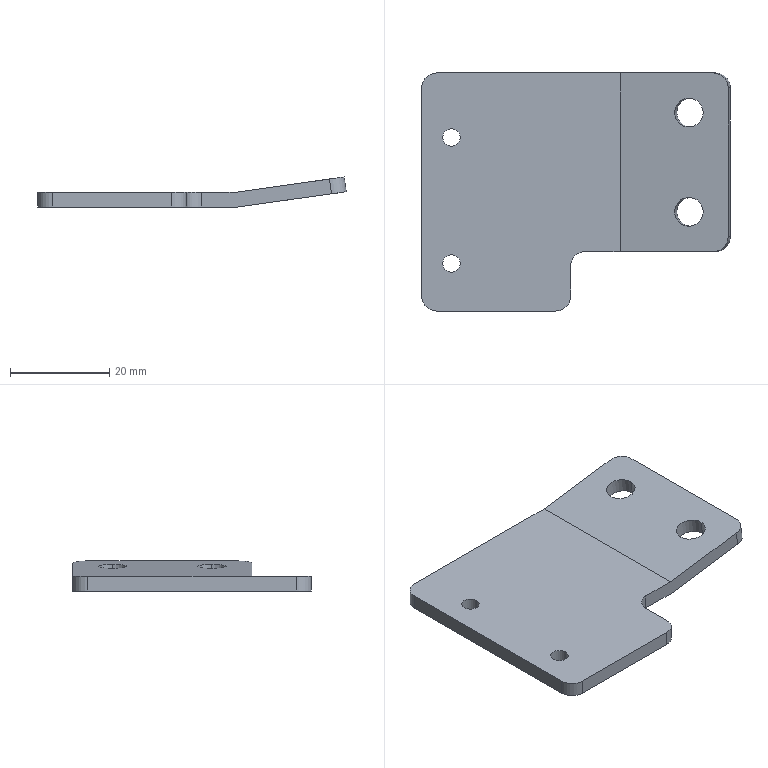Part | STEP file | J014-EBZ05-21-06 | 1 solid | 24 faces | box 62.203 x 48 x 6.062 mm | volume 7559 mm3 | cylinder 14 | plane 10 | commonest cylinder face diameters 6 x6 3.5 x4 5.8 x4
STEP:
#1=CARTESIAN_POINT('',(50.992,20.,4.545));
#2=VERTEX_POINT('',#1);
#3=CARTESIAN_POINT('',(56.736,20.,5.352));
#4=VERTEX_POINT('',#3);
#5=CARTESIAN_POINT('',(53.864,20.,4.948));
#6=DIRECTION('',(0.1392,0.,-0.9903));
#7=DIRECTION('',(0.9903,0.,0.1392));
#8=AXIS2_PLACEMENT_3D('',#5,#6,#7);
#9=CIRCLE('',#8,2.9);
#10=EDGE_CURVE('',#2,#4,#9,.T.);
#11=ORIENTED_EDGE('',*,*,#10,.F.);
#12=CARTESIAN_POINT('',(51.409,20.,1.574));
#13=VERTEX_POINT('',#12);
#14=CARTESIAN_POINT('',(50.992,20.,4.545));
#15=DIRECTION('',(0.1392,0.,-0.9903));
#16=VECTOR('',#15,1000.);
#17=LINE('',#14,#16);
#18=EDGE_CURVE('',#2,#13,#17,.T.);
#19=ORIENTED_EDGE('',*,*,#18,.T.);
#20=CARTESIAN_POINT('',(57.153,20.,2.381));
#21=VERTEX_POINT('',#20);
#22=CARTESIAN_POINT('',(54.281,20.,1.978));
#23=DIRECTION('',(-0.1392,0.,0.9903));
#24=DIRECTION('',(-0.9903,0.,-0.1392));
#25=AXIS2_PLACEMENT_3D('',#22,#23,#24);
#26=CIRCLE('',#25,2.9);
#27=EDGE_CURVE('',#21,#13,#26,.T.);
#28=ORIENTED_EDGE('',*,*,#27,.F.);
#29=CARTESIAN_POINT('',(56.736,20.,5.352));
#30=DIRECTION('',(0.1392,0.,-0.9903));
#31=VECTOR('',#30,1000.);
#32=LINE('',#29,#31);
#33=EDGE_CURVE('',#4,#21,#32,.T.);
#34=ORIENTED_EDGE('',*,*,#33,.F.);
#35=EDGE_LOOP('',(#11,#19,#28,#34));
#36=FACE_OUTER_BOUND('',#35,.T.);
#37=CARTESIAN_POINT('',(53.864,20.,4.948));
#38=DIRECTION('',(0.1392,0.,-0.9903));
#39=DIRECTION('',(0.9903,0.,0.1392));
#40=AXIS2_PLACEMENT_3D('',#37,#38,#39);
#41=CYLINDRICAL_SURFACE('',#40,2.9);
#42=ADVANCED_FACE('',(#36),#41,.F.);
#43=CARTESIAN_POINT('',(50.992,40.,4.545));
#44=VERTEX_POINT('',#43);
#45=CARTESIAN_POINT('',(56.736,40.,5.352));
#46=VERTEX_POINT('',#45);
#47=CARTESIAN_POINT('',(53.864,40.,4.948));
#48=DIRECTION('',(0.1392,0.,-0.9903));
#49=DIRECTION('',(0.9903,0.,0.1392));
#50=AXIS2_PLACEMENT_3D('',#47,#48,#49);
#51=CIRCLE('',#50,2.9);
#52=EDGE_CURVE('',#44,#46,#51,.T.);
#53=ORIENTED_EDGE('',*,*,#52,.F.);
#54=CARTESIAN_POINT('',(51.409,40.,1.574));
#55=VERTEX_POINT('',#54);
#56=CARTESIAN_POINT('',(50.992,40.,4.545));
#57=DIRECTION('',(0.1392,0.,-0.9903));
#58=VECTOR('',#57,1000.);
#59=LINE('',#56,#58);
#60=EDGE_CURVE('',#44,#55,#59,.T.);
#61=ORIENTED_EDGE('',*,*,#60,.T.);
#62=CARTESIAN_POINT('',(57.153,40.,2.381));
#63=VERTEX_POINT('',#62);
#64=CARTESIAN_POINT('',(54.281,40.,1.978));
#65=DIRECTION('',(-0.1392,0.,0.9903));
#66=DIRECTION('',(-0.9903,0.,-0.1392));
#67=AXIS2_PLACEMENT_3D('',#64,#65,#66);
#68=CIRCLE('',#67,2.9);
#69=EDGE_CURVE('',#63,#55,#68,.T.);
#70=ORIENTED_EDGE('',*,*,#69,.F.);
#71=CARTESIAN_POINT('',(56.736,40.,5.352));
#72=DIRECTION('',(0.1392,0.,-0.9903));
#73=VECTOR('',#72,1000.);
#74=LINE('',#71,#73);
#75=EDGE_CURVE('',#46,#63,#74,.T.);
#76=ORIENTED_EDGE('',*,*,#75,.F.);
#77=EDGE_LOOP('',(#53,#61,#70,#76));
#78=FACE_OUTER_BOUND('',#77,.T.);
#79=CARTESIAN_POINT('',(53.864,40.,4.948));
#80=DIRECTION('',(0.1392,0.,-0.9903));
#81=DIRECTION('',(0.9903,0.,0.1392));
#82=AXIS2_PLACEMENT_3D('',#79,#80,#81);
#83=CYLINDRICAL_SURFACE('',#82,2.9);
#84=ADVANCED_FACE('',(#78),#83,.F.);
#85=CARTESIAN_POINT('',(4.25,9.6,3.));
#86=VERTEX_POINT('',#85);
#87=CARTESIAN_POINT('',(7.75,9.6,3.));
#88=VERTEX_POINT('',#87);
#89=CARTESIAN_POINT('',(6.,9.6,3.));
#90=DIRECTION('',(0.,0.,-1.));
#91=DIRECTION('',(1.,0.,0.));
#92=AXIS2_PLACEMENT_3D('',#89,#90,#91);
#93=CIRCLE('',#92,1.75);
#94=EDGE_CURVE('',#86,#88,#93,.T.);
#95=ORIENTED_EDGE('',*,*,#94,.F.);
#96=CARTESIAN_POINT('',(4.25,9.6,0.));
#97=VERTEX_POINT('',#96);
#98=CARTESIAN_POINT('',(4.25,9.6,3.));
#99=DIRECTION('',(0.,0.,-1.));
#100=VECTOR('',#99,1000.);
#101=LINE('',#98,#100);
#102=EDGE_CURVE('',#86,#97,#101,.T.);
#103=ORIENTED_EDGE('',*,*,#102,.T.);
#104=CARTESIAN_POINT('',(7.75,9.6,0.));
#105=VERTEX_POINT('',#104);
#106=CARTESIAN_POINT('',(6.,9.6,0.));
#107=DIRECTION('',(0.,0.,1.));
#108=DIRECTION('',(-1.,0.,0.));
#109=AXIS2_PLACEMENT_3D('',#106,#107,#108);
#110=CIRCLE('',#109,1.75);
#111=EDGE_CURVE('',#105,#97,#110,.T.);
#112=ORIENTED_EDGE('',*,*,#111,.F.);
#113=CARTESIAN_POINT('',(7.75,9.6,3.));
#114=DIRECTION('',(0.,0.,-1.));
#115=VECTOR('',#114,1000.);
#116=LINE('',#113,#115);
#117=EDGE_CURVE('',#88,#105,#116,.T.);
#118=ORIENTED_EDGE('',*,*,#117,.F.);
#119=EDGE_LOOP('',(#95,#103,#112,#118));
#120=FACE_OUTER_BOUND('',#119,.T.);
#121=CARTESIAN_POINT('',(6.,9.6,3.));
#122=DIRECTION('',(0.,0.,-1.));
#123=DIRECTION('',(1.,0.,0.));
#124=AXIS2_PLACEMENT_3D('',#121,#122,#123);
#125=CYLINDRICAL_SURFACE('',#124,1.75);
#126=ADVANCED_FACE('',(#120),#125,.F.);
#127=CARTESIAN_POINT('',(4.25,35.,3.));
#128=VERTEX_POINT('',#127);
#129=CARTESIAN_POINT('',(7.75,35.,3.));
#130=VERTEX_POINT('',#129);
#131=CARTESIAN_POINT('',(6.,35.,3.));
#132=DIRECTION('',(0.,0.,-1.));
#133=DIRECTION('',(1.,0.,0.));
#134=AXIS2_PLACEMENT_3D('',#131,#132,#133);
#135=CIRCLE('',#134,1.75);
#136=EDGE_CURVE('',#128,#130,#135,.T.);
#137=ORIENTED_EDGE('',*,*,#136,.F.);
#138=CARTESIAN_POINT('',(4.25,35.,0.));
#139=VERTEX_POINT('',#138);
#140=CARTESIAN_POINT('',(4.25,35.,3.));
#141=DIRECTION('',(0.,0.,-1.));
#142=VECTOR('',#141,1000.);
#143=LINE('',#140,#142);
#144=EDGE_CURVE('',#128,#139,#143,.T.);
#145=ORIENTED_EDGE('',*,*,#144,.T.);
#146=CARTESIAN_POINT('',(7.75,35.,0.));
#147=VERTEX_POINT('',#146);
#148=CARTESIAN_POINT('',(6.,35.,0.));
#149=DIRECTION('',(0.,0.,1.));
#150=DIRECTION('',(-1.,0.,0.));
#151=AXIS2_PLACEMENT_3D('',#148,#149,#150);
#152=CIRCLE('',#151,1.75);
#153=EDGE_CURVE('',#147,#139,#152,.T.);
#154=ORIENTED_EDGE('',*,*,#153,.F.);
#155=CARTESIAN_POINT('',(7.75,35.,3.));
#156=DIRECTION('',(0.,0.,-1.));
#157=VECTOR('',#156,1000.);
#158=LINE('',#155,#157);
#159=EDGE_CURVE('',#130,#147,#158,.T.);
#160=ORIENTED_EDGE('',*,*,#159,.F.);
#161=EDGE_LOOP('',(#137,#145,#154,#160));
#162=FACE_OUTER_BOUND('',#161,.T.);
#163=CARTESIAN_POINT('',(6.,35.,3.));
#164=DIRECTION('',(0.,0.,-1.));
#165=DIRECTION('',(1.,0.,0.));
#166=AXIS2_PLACEMENT_3D('',#163,#164,#165);
#167=CYLINDRICAL_SURFACE('',#166,1.75);
#168=ADVANCED_FACE('',(#162),#167,.F.);
#169=CARTESIAN_POINT('',(61.786,45.,6.062));
#170=VERTEX_POINT('',#169);
#171=CARTESIAN_POINT('',(61.786,15.,6.062));
#172=VERTEX_POINT('',#171);
#173=CARTESIAN_POINT('',(61.786,24.,6.062));
#174=DIRECTION('',(0.,-1.,0.));
#175=VECTOR('',#174,1000.);
#176=LINE('',#173,#175);
#177=EDGE_CURVE('',#170,#172,#176,.T.);
#178=ORIENTED_EDGE('',*,*,#177,.T.);
#179=CARTESIAN_POINT('',(62.203,15.,3.091));
#180=VERTEX_POINT('',#179);
#181=CARTESIAN_POINT('',(62.203,15.,3.091));
#182=DIRECTION('',(0.1392,0.,-0.9903));
#183=VECTOR('',#182,1000.);
#184=LINE('',#181,#183);
#185=EDGE_CURVE('',#172,#180,#184,.T.);
#186=ORIENTED_EDGE('',*,*,#185,.T.);
#187=CARTESIAN_POINT('',(62.203,45.,3.091));
#188=VERTEX_POINT('',#187);
#189=CARTESIAN_POINT('',(62.203,24.,3.091));
#190=DIRECTION('',(0.,1.,0.));
#191=VECTOR('',#190,1000.);
#192=LINE('',#189,#191);
#193=EDGE_CURVE('',#180,#188,#192,.T.);
#194=ORIENTED_EDGE('',*,*,#193,.T.);
#195=CARTESIAN_POINT('',(61.786,45.,6.062));
#196=DIRECTION('',(-0.1392,0.,0.9903));
#197=VECTOR('',#196,1000.);
#198=LINE('',#195,#197);
#199=EDGE_CURVE('',#188,#170,#198,.T.);
#200=ORIENTED_EDGE('',*,*,#199,.T.);
#201=EDGE_LOOP('',(#178,#186,#194,#200));
#202=FACE_OUTER_BOUND('',#201,.T.);
#203=CARTESIAN_POINT('',(61.786,24.,6.062));
#204=DIRECTION('',(0.9903,0.,0.1392));
#205=DIRECTION('',(-0.1392,0.,0.9903));
#206=AXIS2_PLACEMENT_3D('',#203,#204,#205);
#207=PLANE('',#206);
#208=ADVANCED_FACE('',(#202),#207,.T.);
#209=ORIENTED_EDGE('',*,*,#193,.F.);
#210=CARTESIAN_POINT('',(59.233,12.,2.673));
#211=VERTEX_POINT('',#210);
#212=CARTESIAN_POINT('',(59.233,15.,2.673));
#213=DIRECTION('',(0.1392,0.,-0.9903));
#214=DIRECTION('',(0.,-1.,0.));
#215=AXIS2_PLACEMENT_3D('',#212,#213,#214);
#216=CIRCLE('',#215,3.);
#217=EDGE_CURVE('',#180,#211,#216,.T.);
#218=ORIENTED_EDGE('',*,*,#217,.T.);
#219=CARTESIAN_POINT('',(40.21,12.,0.));
#220=VERTEX_POINT('',#219);
#221=CARTESIAN_POINT('',(50.32,12.,1.421));
#222=DIRECTION('',(0.9903,0.,0.1392));
#223=VECTOR('',#222,1000.);
#224=LINE('',#221,#223);
#225=EDGE_CURVE('',#220,#211,#224,.T.);
#226=ORIENTED_EDGE('',*,*,#225,.F.);
#227=CARTESIAN_POINT('',(40.21,48.,0.));
#228=VERTEX_POINT('',#227);
#229=CARTESIAN_POINT('',(40.21,24.,0.));
#230=DIRECTION('',(0.,1.,0.));
#231=VECTOR('',#230,1000.);
#232=LINE('',#229,#231);
#233=EDGE_CURVE('',#220,#228,#232,.T.);
#234=ORIENTED_EDGE('',*,*,#233,.T.);
#235=CARTESIAN_POINT('',(59.233,48.,2.673));
#236=VERTEX_POINT('',#235);
#237=CARTESIAN_POINT('',(50.32,48.,1.421));
#238=DIRECTION('',(-0.9903,0.,-0.1392));
#239=VECTOR('',#238,1000.);
#240=LINE('',#237,#239);
#241=EDGE_CURVE('',#236,#228,#240,.T.);
#242=ORIENTED_EDGE('',*,*,#241,.F.);
#243=CARTESIAN_POINT('',(59.233,45.,2.673));
#244=DIRECTION('',(0.1392,0.,-0.9903));
#245=DIRECTION('',(0.,-1.,0.));
#246=AXIS2_PLACEMENT_3D('',#243,#244,#245);
#247=CIRCLE('',#246,3.);
#248=EDGE_CURVE('',#236,#188,#247,.T.);
#249=ORIENTED_EDGE('',*,*,#248,.T.);
#250=EDGE_LOOP('',(#209,#218,#226,#234,#242,#249));
#251=FACE_OUTER_BOUND('',#250,.T.);
#252=ORIENTED_EDGE('',*,*,#27,.T.);
#253=CARTESIAN_POINT('',(54.281,20.,1.978));
#254=DIRECTION('',(-0.1392,0.,0.9903));
#255=DIRECTION('',(-0.9903,0.,-0.1392));
#256=AXIS2_PLACEMENT_3D('',#253,#254,#255);
#257=CIRCLE('',#256,2.9);
#258=EDGE_CURVE('',#13,#21,#257,.T.);
#259=ORIENTED_EDGE('',*,*,#258,.T.);
#260=EDGE_LOOP('',(#252,#259));
#261=FACE_BOUND('',#260,.T.);
#262=ORIENTED_EDGE('',*,*,#69,.T.);
#263=CARTESIAN_POINT('',(54.281,40.,1.978));
#264=DIRECTION('',(-0.1392,0.,0.9903));
#265=DIRECTION('',(-0.9903,0.,-0.1392));
#266=AXIS2_PLACEMENT_3D('',#263,#264,#265);
#267=CIRCLE('',#266,2.9);
#268=EDGE_CURVE('',#55,#63,#267,.T.);
#269=ORIENTED_EDGE('',*,*,#268,.T.);
#270=EDGE_LOOP('',(#262,#269));
#271=FACE_BOUND('',#270,.T.);
#272=CARTESIAN_POINT('',(50.32,24.,1.421));
#273=DIRECTION('',(0.1392,0.,-0.9903));
#274=DIRECTION('',(0.,-1.,0.));
#275=AXIS2_PLACEMENT_3D('',#272,#273,#274);
#276=PLANE('',#275);
#277=ADVANCED_FACE('',(#251,#261,#271),#276,.T.);
#278=CARTESIAN_POINT('',(3.,48.,0.));
#279=VERTEX_POINT('',#278);
#280=CARTESIAN_POINT('',(49.903,48.,0.));
#281=DIRECTION('',(-1.,0.,0.));
#282=VECTOR('',#281,1000.);
#283=LINE('',#280,#282);
#284=EDGE_CURVE('',#228,#279,#283,.T.);
#285=ORIENTED_EDGE('',*,*,#284,.T.);
#286=CARTESIAN_POINT('',(3.,48.,3.));
#287=VERTEX_POINT('',#286);
#288=CARTESIAN_POINT('',(3.,48.,4.392));
#289=DIRECTION('',(0.,0.,1.));
#290=VECTOR('',#289,1000.);
#291=LINE('',#288,#290);
#292=EDGE_CURVE('',#279,#287,#291,.T.);
#293=ORIENTED_EDGE('',*,*,#292,.T.);
#294=CARTESIAN_POINT('',(40.,48.,3.));
#295=VERTEX_POINT('',#294);
#296=CARTESIAN_POINT('',(20.,48.,3.));
#297=DIRECTION('',(1.,0.,0.));
#298=VECTOR('',#297,1000.);
#299=LINE('',#296,#298);
#300=EDGE_CURVE('',#287,#295,#299,.T.);
#301=ORIENTED_EDGE('',*,*,#300,.T.);
#302=CARTESIAN_POINT('',(58.815,48.,5.644));
#303=VERTEX_POINT('',#302);
#304=CARTESIAN_POINT('',(49.903,48.,4.392));
#305=DIRECTION('',(0.9903,0.,0.1392));
#306=VECTOR('',#305,1000.);
#307=LINE('',#304,#306);
#308=EDGE_CURVE('',#295,#303,#307,.T.);
#309=ORIENTED_EDGE('',*,*,#308,.T.);
#310=CARTESIAN_POINT('',(58.815,48.,5.644));
#311=DIRECTION('',(0.1392,0.,-0.9903));
#312=VECTOR('',#311,1000.);
#313=LINE('',#310,#312);
#314=EDGE_CURVE('',#303,#236,#313,.T.);
#315=ORIENTED_EDGE('',*,*,#314,.T.);
#316=ORIENTED_EDGE('',*,*,#241,.T.);
#317=EDGE_LOOP('',(#285,#293,#301,#309,#315,#316));
#318=FACE_OUTER_BOUND('',#317,.T.);
#319=CARTESIAN_POINT('',(49.903,48.,4.392));
#320=DIRECTION('',(0.,1.,0.));
#321=DIRECTION('',(0.1392,0.,-0.9903));
#322=AXIS2_PLACEMENT_3D('',#319,#320,#321);
#323=PLANE('',#322);
#324=ADVANCED_FACE('',(#318),#323,.T.);
#325=CARTESIAN_POINT('',(3.,0.,0.));
#326=VERTEX_POINT('',#325);
#327=CARTESIAN_POINT('',(27.,0.,0.));
#328=VERTEX_POINT('',#327);
#329=CARTESIAN_POINT('',(49.903,0.,0.));
#330=DIRECTION('',(1.,0.,0.));
#331=VECTOR('',#330,1000.);
#332=LINE('',#329,#331);
#333=EDGE_CURVE('',#326,#328,#332,.T.);
#334=ORIENTED_EDGE('',*,*,#333,.T.);
#335=CARTESIAN_POINT('',(27.,0.,3.));
#336=VERTEX_POINT('',#335);
#337=CARTESIAN_POINT('',(27.,0.,3.));
#338=DIRECTION('',(0.,0.,1.));
#339=VECTOR('',#338,1000.);
#340=LINE('',#337,#339);
#341=EDGE_CURVE('',#328,#336,#340,.T.);
#342=ORIENTED_EDGE('',*,*,#341,.T.);
#343=CARTESIAN_POINT('',(3.,0.,3.));
#344=VERTEX_POINT('',#343);
#345=CARTESIAN_POINT('',(20.,0.,3.));
#346=DIRECTION('',(-1.,0.,0.));
#347=VECTOR('',#346,1000.);
#348=LINE('',#345,#347);
#349=EDGE_CURVE('',#336,#344,#348,.T.);
#350=ORIENTED_EDGE('',*,*,#349,.T.);
#351=CARTESIAN_POINT('',(3.,0.,4.392));
#352=DIRECTION('',(0.,0.,-1.));
#353=VECTOR('',#352,1000.);
#354=LINE('',#351,#353);
#355=EDGE_CURVE('',#344,#326,#354,.T.);
#356=ORIENTED_EDGE('',*,*,#355,.T.);
#357=EDGE_LOOP('',(#334,#342,#350,#356));
#358=FACE_OUTER_BOUND('',#357,.T.);
#359=CARTESIAN_POINT('',(49.903,0.,4.392));
#360=DIRECTION('',(0.,-1.,0.));
#361=DIRECTION('',(-0.1392,0.,0.9903));
#362=AXIS2_PLACEMENT_3D('',#359,#360,#361);
#363=PLANE('',#362);
#364=ADVANCED_FACE('',(#358),#363,.T.);
#365=CARTESIAN_POINT('',(58.815,12.,5.644));
#366=VERTEX_POINT('',#365);
#367=CARTESIAN_POINT('',(40.,12.,3.));
#368=VERTEX_POINT('',#367);
#369=CARTESIAN_POINT('',(49.903,12.,4.392));
#370=DIRECTION('',(-0.9903,0.,-0.1392));
#371=VECTOR('',#370,1000.);
#372=LINE('',#369,#371);
#373=EDGE_CURVE('',#366,#368,#372,.T.);
#374=ORIENTED_EDGE('',*,*,#373,.F.);
#375=CARTESIAN_POINT('',(58.815,15.,5.644));
#376=DIRECTION('',(-0.1392,0.,0.9903));
#377=DIRECTION('',(0.,1.,0.));
#378=AXIS2_PLACEMENT_3D('',#375,#376,#377);
#379=CIRCLE('',#378,3.);
#380=EDGE_CURVE('',#366,#172,#379,.T.);
#381=ORIENTED_EDGE('',*,*,#380,.T.);
#382=ORIENTED_EDGE('',*,*,#177,.F.);
#383=CARTESIAN_POINT('',(58.815,45.,5.644));
#384=DIRECTION('',(-0.1392,0.,0.9903));
#385=DIRECTION('',(0.,1.,0.));
#386=AXIS2_PLACEMENT_3D('',#383,#384,#385);
#387=CIRCLE('',#386,3.);
#388=EDGE_CURVE('',#170,#303,#387,.T.);
#389=ORIENTED_EDGE('',*,*,#388,.T.);
#390=ORIENTED_EDGE('',*,*,#308,.F.);
#391=CARTESIAN_POINT('',(40.,24.,3.));
#392=DIRECTION('',(0.,-1.,0.));
#393=VECTOR('',#392,1000.);
#394=LINE('',#391,#393);
#395=EDGE_CURVE('',#295,#368,#394,.T.);
#396=ORIENTED_EDGE('',*,*,#395,.T.);
#397=EDGE_LOOP('',(#374,#381,#382,#389,#390,#396));
#398=FACE_OUTER_BOUND('',#397,.T.);
#399=CARTESIAN_POINT('',(53.864,20.,4.948));
#400=DIRECTION('',(0.1392,0.,-0.9903));
#401=DIRECTION('',(0.9903,0.,0.1392));
#402=AXIS2_PLACEMENT_3D('',#399,#400,#401);
#403=CIRCLE('',#402,2.9);
#404=EDGE_CURVE('',#4,#2,#403,.T.);
#405=ORIENTED_EDGE('',*,*,#404,.T.);
#406=ORIENTED_EDGE('',*,*,#10,.T.);
#407=EDGE_LOOP('',(#405,#406));
#408=FACE_BOUND('',#407,.T.);
#409=CARTESIAN_POINT('',(53.864,40.,4.948));
#410=DIRECTION('',(0.1392,0.,-0.9903));
#411=DIRECTION('',(0.9903,0.,0.1392));
#412=AXIS2_PLACEMENT_3D('',#409,#410,#411);
#413=CIRCLE('',#412,2.9);
#414=EDGE_CURVE('',#46,#44,#413,.T.);
#415=ORIENTED_EDGE('',*,*,#414,.T.);
#416=ORIENTED_EDGE('',*,*,#52,.T.);
#417=EDGE_LOOP('',(#415,#416));
#418=FACE_BOUND('',#417,.T.);
#419=CARTESIAN_POINT('',(49.903,24.,4.392));
#420=DIRECTION('',(-0.1392,0.,0.9903));
#421=DIRECTION('',(0.,1.,0.));
#422=AXIS2_PLACEMENT_3D('',#419,#420,#421);
#423=PLANE('',#422);
#424=ADVANCED_FACE('',(#398,#408,#418),#423,.T.);
#425=CARTESIAN_POINT('',(30.,3.,0.));
#426=VERTEX_POINT('',#425);
#427=CARTESIAN_POINT('',(30.,9.,0.));
#428=VERTEX_POINT('',#427);
#429=CARTESIAN_POINT('',(30.,59.004,0.));
#430=DIRECTION('',(0.,1.,0.));
#431=VECTOR('',#430,1000.);
#432=LINE('',#429,#431);
#433=EDGE_CURVE('',#426,#428,#432,.T.);
#434=ORIENTED_EDGE('',*,*,#433,.F.);
#435=CARTESIAN_POINT('',(27.,3.,0.));
#436=DIRECTION('',(0.,0.,-1.));
#437=DIRECTION('',(1.,0.,0.));
#438=AXIS2_PLACEMENT_3D('',#435,#436,#437);
#439=CIRCLE('',#438,3.);
#440=EDGE_CURVE('',#426,#328,#439,.T.);
#441=ORIENTED_EDGE('',*,*,#440,.T.);
#442=ORIENTED_EDGE('',*,*,#333,.F.);
#443=CARTESIAN_POINT('',(0.,3.,0.));
#444=VERTEX_POINT('',#443);
#445=CARTESIAN_POINT('',(3.,3.,0.));
#446=DIRECTION('',(0.,0.,-1.));
#447=DIRECTION('',(1.,0.,0.));
#448=AXIS2_PLACEMENT_3D('',#445,#446,#447);
#449=CIRCLE('',#448,3.);
#450=EDGE_CURVE('',#326,#444,#449,.T.);
#451=ORIENTED_EDGE('',*,*,#450,.T.);
#452=CARTESIAN_POINT('',(0.,45.,0.));
#453=VERTEX_POINT('',#452);
#454=CARTESIAN_POINT('',(0.,24.,0.));
#455=DIRECTION('',(0.,-1.,0.));
#456=VECTOR('',#455,1000.);
#457=LINE('',#454,#456);
#458=EDGE_CURVE('',#453,#444,#457,.T.);
#459=ORIENTED_EDGE('',*,*,#458,.F.);
#460=CARTESIAN_POINT('',(3.,45.,0.));
#461=DIRECTION('',(0.,0.,-1.));
#462=DIRECTION('',(1.,0.,0.));
#463=AXIS2_PLACEMENT_3D('',#460,#461,#462);
#464=CIRCLE('',#463,3.);
#465=EDGE_CURVE('',#453,#279,#464,.T.);
#466=ORIENTED_EDGE('',*,*,#465,.T.);
#467=ORIENTED_EDGE('',*,*,#284,.F.);
#468=ORIENTED_EDGE('',*,*,#233,.F.);
#469=CARTESIAN_POINT('',(33.,12.,0.));
#470=VERTEX_POINT('',#469);
#471=CARTESIAN_POINT('',(55.128,12.,0.));
#472=DIRECTION('',(1.,0.,0.));
#473=VECTOR('',#472,1000.);
#474=LINE('',#471,#473);
#475=EDGE_CURVE('',#470,#220,#474,.T.);
#476=ORIENTED_EDGE('',*,*,#475,.F.);
#477=CARTESIAN_POINT('',(33.,9.,0.));
#478=DIRECTION('',(0.,0.,1.));
#479=DIRECTION('',(1.,0.,0.));
#480=AXIS2_PLACEMENT_3D('',#477,#478,#479);
#481=CIRCLE('',#480,3.);
#482=EDGE_CURVE('',#470,#428,#481,.T.);
#483=ORIENTED_EDGE('',*,*,#482,.T.);
#484=EDGE_LOOP('',(#434,#441,#442,#451,#459,#466,#467,#468,#476,#483));
#485=FACE_OUTER_BOUND('',#484,.T.);
#486=ORIENTED_EDGE('',*,*,#111,.T.);
#487=CARTESIAN_POINT('',(6.,9.6,0.));
#488=DIRECTION('',(0.,0.,1.));
#489=DIRECTION('',(-1.,0.,0.));
#490=AXIS2_PLACEMENT_3D('',#487,#488,#489);
#491=CIRCLE('',#490,1.75);
#492=EDGE_CURVE('',#97,#105,#491,.T.);
#493=ORIENTED_EDGE('',*,*,#492,.T.);
#494=EDGE_LOOP('',(#486,#493));
#495=FACE_BOUND('',#494,.T.);
#496=ORIENTED_EDGE('',*,*,#153,.T.);
#497=CARTESIAN_POINT('',(6.,35.,0.));
#498=DIRECTION('',(0.,0.,1.));
#499=DIRECTION('',(-1.,0.,0.));
#500=AXIS2_PLACEMENT_3D('',#497,#498,#499);
#501=CIRCLE('',#500,1.75);
#502=EDGE_CURVE('',#139,#147,#501,.T.);
#503=ORIENTED_EDGE('',*,*,#502,.T.);
#504=EDGE_LOOP('',(#496,#503));
#505=FACE_BOUND('',#504,.T.);
#506=CARTESIAN_POINT('',(55.128,59.004,0.));
#507=DIRECTION('',(0.,0.,-1.));
#508=DIRECTION('',(0.8411,0.5409,0.));
#509=AXIS2_PLACEMENT_3D('',#506,#507,#508);
#510=PLANE('',#509);
#511=ADVANCED_FACE('',(#485,#495,#505),#510,.T.);
#512=ORIENTED_EDGE('',*,*,#458,.T.);
#513=CARTESIAN_POINT('',(0.,3.,3.));
#514=VERTEX_POINT('',#513);
#515=CARTESIAN_POINT('',(0.,3.,3.));
#516=DIRECTION('',(0.,0.,1.));
#517=VECTOR('',#516,1000.);
#518=LINE('',#515,#517);
#519=EDGE_CURVE('',#444,#514,#518,.T.);
#520=ORIENTED_EDGE('',*,*,#519,.T.);
#521=CARTESIAN_POINT('',(0.,45.,3.));
#522=VERTEX_POINT('',#521);
#523=CARTESIAN_POINT('',(0.,24.,3.));
#524=DIRECTION('',(0.,1.,0.));
#525=VECTOR('',#524,1000.);
#526=LINE('',#523,#525);
#527=EDGE_CURVE('',#514,#522,#526,.T.);
#528=ORIENTED_EDGE('',*,*,#527,.T.);
#529=CARTESIAN_POINT('',(0.,45.,3.));
#530=DIRECTION('',(0.,0.,-1.));
#531=VECTOR('',#530,1000.);
#532=LINE('',#529,#531);
#533=EDGE_CURVE('',#522,#453,#532,.T.);
#534=ORIENTED_EDGE('',*,*,#533,.T.);
#535=EDGE_LOOP('',(#512,#520,#528,#534));
#536=FACE_OUTER_BOUND('',#535,.T.);
#537=CARTESIAN_POINT('',(0.,24.,3.));
#538=DIRECTION('',(-1.,0.,0.));
#539=DIRECTION('',(0.,0.,-1.));
#540=AXIS2_PLACEMENT_3D('',#537,#538,#539);
#541=PLANE('',#540);
#542=ADVANCED_FACE('',(#536),#541,.T.);
#543=ORIENTED_EDGE('',*,*,#349,.F.);
#544=CARTESIAN_POINT('',(30.,3.,3.));
#545=VERTEX_POINT('',#544);
#546=CARTESIAN_POINT('',(27.,3.,3.));
#547=DIRECTION('',(0.,0.,1.));
#548=DIRECTION('',(-1.,0.,0.));
#549=AXIS2_PLACEMENT_3D('',#546,#547,#548);
#550=CIRCLE('',#549,3.);
#551=EDGE_CURVE('',#336,#545,#550,.T.);
#552=ORIENTED_EDGE('',*,*,#551,.T.);
#553=CARTESIAN_POINT('',(30.,9.,3.));
#554=VERTEX_POINT('',#553);
#555=CARTESIAN_POINT('',(30.,24.,3.));
#556=DIRECTION('',(0.,-1.,0.));
#557=VECTOR('',#556,1000.);
#558=LINE('',#555,#557);
#559=EDGE_CURVE('',#554,#545,#558,.T.);
#560=ORIENTED_EDGE('',*,*,#559,.F.);
#561=CARTESIAN_POINT('',(33.,12.,3.));
#562=VERTEX_POINT('',#561);
#563=CARTESIAN_POINT('',(33.,9.,3.));
#564=DIRECTION('',(0.,0.,-1.));
#565=DIRECTION('',(-1.,0.,0.));
#566=AXIS2_PLACEMENT_3D('',#563,#564,#565);
#567=CIRCLE('',#566,3.);
#568=EDGE_CURVE('',#554,#562,#567,.T.);
#569=ORIENTED_EDGE('',*,*,#568,.T.);
#570=CARTESIAN_POINT('',(20.,12.,3.));
#571=DIRECTION('',(-1.,0.,0.));
#572=VECTOR('',#571,1000.);
#573=LINE('',#570,#572);
#574=EDGE_CURVE('',#368,#562,#573,.T.);
#575=ORIENTED_EDGE('',*,*,#574,.F.);
#576=ORIENTED_EDGE('',*,*,#395,.F.);
#577=ORIENTED_EDGE('',*,*,#300,.F.);
#578=CARTESIAN_POINT('',(3.,45.,3.));
#579=DIRECTION('',(0.,0.,1.));
#580=DIRECTION('',(-1.,0.,0.));
#581=AXIS2_PLACEMENT_3D('',#578,#579,#580);
#582=CIRCLE('',#581,3.);
#583=EDGE_CURVE('',#287,#522,#582,.T.);
#584=ORIENTED_EDGE('',*,*,#583,.T.);
#585=ORIENTED_EDGE('',*,*,#527,.F.);
#586=CARTESIAN_POINT('',(3.,3.,3.));
#587=DIRECTION('',(0.,0.,1.));
#588=DIRECTION('',(-1.,0.,0.));
#589=AXIS2_PLACEMENT_3D('',#586,#587,#588);
#590=CIRCLE('',#589,3.);
#591=EDGE_CURVE('',#514,#344,#590,.T.);
#592=ORIENTED_EDGE('',*,*,#591,.T.);
#593=EDGE_LOOP('',(#543,#552,#560,#569,#575,#576,#577,#584,#585,#592));
#594=FACE_OUTER_BOUND('',#593,.T.);
#595=CARTESIAN_POINT('',(6.,9.6,3.));
#596=DIRECTION('',(0.,0.,-1.));
#597=DIRECTION('',(1.,0.,0.));
#598=AXIS2_PLACEMENT_3D('',#595,#596,#597);
#599=CIRCLE('',#598,1.75);
#600=EDGE_CURVE('',#88,#86,#599,.T.);
#601=ORIENTED_EDGE('',*,*,#600,.T.);
#602=ORIENTED_EDGE('',*,*,#94,.T.);
#603=EDGE_LOOP('',(#601,#602));
#604=FACE_BOUND('',#603,.T.);
#605=CARTESIAN_POINT('',(6.,35.,3.));
#606=DIRECTION('',(0.,0.,-1.));
#607=DIRECTION('',(1.,0.,0.));
#608=AXIS2_PLACEMENT_3D('',#605,#606,#607);
#609=CIRCLE('',#608,1.75);
#610=EDGE_CURVE('',#130,#128,#609,.T.);
#611=ORIENTED_EDGE('',*,*,#610,.T.);
#612=ORIENTED_EDGE('',*,*,#136,.T.);
#613=EDGE_LOOP('',(#611,#612));
#614=FACE_BOUND('',#613,.T.);
#615=CARTESIAN_POINT('',(20.,24.,3.));
#616=DIRECTION('',(0.,0.,1.));
#617=DIRECTION('',(0.,1.,0.));
#618=AXIS2_PLACEMENT_3D('',#615,#616,#617);
#619=PLANE('',#618);
#620=ADVANCED_FACE('',(#594,#604,#614),#619,.T.);
#621=ORIENTED_EDGE('',*,*,#388,.F.);
#622=ORIENTED_EDGE('',*,*,#199,.F.);
#623=ORIENTED_EDGE('',*,*,#248,.F.);
#624=ORIENTED_EDGE('',*,*,#314,.F.);
#625=EDGE_LOOP('',(#621,#622,#623,#624));
#626=FACE_OUTER_BOUND('',#625,.T.);
#627=CARTESIAN_POINT('',(58.815,45.,5.644));
#628=DIRECTION('',(0.1392,0.,-0.9903));
#629=DIRECTION('',(0.,-1.,0.));
#630=AXIS2_PLACEMENT_3D('',#627,#628,#629);
#631=CYLINDRICAL_SURFACE('',#630,3.);
#632=ADVANCED_FACE('',(#626),#631,.T.);
#633=ORIENTED_EDGE('',*,*,#591,.F.);
#634=ORIENTED_EDGE('',*,*,#519,.F.);
#635=ORIENTED_EDGE('',*,*,#450,.F.);
#636=ORIENTED_EDGE('',*,*,#355,.F.);
#637=EDGE_LOOP('',(#633,#634,#635,#636));
#638=FACE_OUTER_BOUND('',#637,.T.);
#639=CARTESIAN_POINT('',(3.,3.,4.392));
#640=DIRECTION('',(0.,0.,-1.));
#641=DIRECTION('',(1.,0.,0.));
#642=AXIS2_PLACEMENT_3D('',#639,#640,#641);
#643=CYLINDRICAL_SURFACE('',#642,3.);
#644=ADVANCED_FACE('',(#638),#643,.T.);
#645=ORIENTED_EDGE('',*,*,#583,.F.);
#646=ORIENTED_EDGE('',*,*,#292,.F.);
#647=ORIENTED_EDGE('',*,*,#465,.F.);
#648=ORIENTED_EDGE('',*,*,#533,.F.);
#649=EDGE_LOOP('',(#645,#646,#647,#648));
#650=FACE_OUTER_BOUND('',#649,.T.);
#651=CARTESIAN_POINT('',(3.,45.,3.));
#652=DIRECTION('',(0.,0.,-1.));
#653=DIRECTION('',(1.,0.,0.));
#654=AXIS2_PLACEMENT_3D('',#651,#652,#653);
#655=CYLINDRICAL_SURFACE('',#654,3.);
#656=ADVANCED_FACE('',(#650),#655,.T.);
#657=ORIENTED_EDGE('',*,*,#144,.F.);
#658=ORIENTED_EDGE('',*,*,#610,.F.);
#659=ORIENTED_EDGE('',*,*,#159,.T.);
#660=ORIENTED_EDGE('',*,*,#502,.F.);
#661=EDGE_LOOP('',(#657,#658,#659,#660));
#662=FACE_OUTER_BOUND('',#661,.T.);
#663=CARTESIAN_POINT('',(6.,35.,3.));
#664=DIRECTION('',(0.,0.,-1.));
#665=DIRECTION('',(1.,0.,0.));
#666=AXIS2_PLACEMENT_3D('',#663,#664,#665);
#667=CYLINDRICAL_SURFACE('',#666,1.75);
#668=ADVANCED_FACE('',(#662),#667,.F.);
#669=ORIENTED_EDGE('',*,*,#102,.F.);
#670=ORIENTED_EDGE('',*,*,#600,.F.);
#671=ORIENTED_EDGE('',*,*,#117,.T.);
#672=ORIENTED_EDGE('',*,*,#492,.F.);
#673=EDGE_LOOP('',(#669,#670,#671,#672));
#674=FACE_OUTER_BOUND('',#673,.T.);
#675=CARTESIAN_POINT('',(6.,9.6,3.));
#676=DIRECTION('',(0.,0.,-1.));
#677=DIRECTION('',(1.,0.,0.));
#678=AXIS2_PLACEMENT_3D('',#675,#676,#677);
#679=CYLINDRICAL_SURFACE('',#678,1.75);
#680=ADVANCED_FACE('',(#674),#679,.F.);
#681=ORIENTED_EDGE('',*,*,#60,.F.);
#682=ORIENTED_EDGE('',*,*,#414,.F.);
#683=ORIENTED_EDGE('',*,*,#75,.T.);
#684=ORIENTED_EDGE('',*,*,#268,.F.);
#685=EDGE_LOOP('',(#681,#682,#683,#684));
#686=FACE_OUTER_BOUND('',#685,.T.);
#687=CARTESIAN_POINT('',(53.864,40.,4.948));
#688=DIRECTION('',(0.1392,0.,-0.9903));
#689=DIRECTION('',(0.9903,0.,0.1392));
#690=AXIS2_PLACEMENT_3D('',#687,#688,#689);
#691=CYLINDRICAL_SURFACE('',#690,2.9);
#692=ADVANCED_FACE('',(#686),#691,.F.);
#693=ORIENTED_EDGE('',*,*,#18,.F.);
#694=ORIENTED_EDGE('',*,*,#404,.F.);
#695=ORIENTED_EDGE('',*,*,#33,.T.);
#696=ORIENTED_EDGE('',*,*,#258,.F.);
#697=EDGE_LOOP('',(#693,#694,#695,#696));
#698=FACE_OUTER_BOUND('',#697,.T.);
#699=CARTESIAN_POINT('',(53.864,20.,4.948));
#700=DIRECTION('',(0.1392,0.,-0.9903));
#701=DIRECTION('',(0.9903,0.,0.1392));
#702=AXIS2_PLACEMENT_3D('',#699,#700,#701);
#703=CYLINDRICAL_SURFACE('',#702,2.9);
#704=ADVANCED_FACE('',(#698),#703,.F.);
#705=ORIENTED_EDGE('',*,*,#574,.T.);
#706=CARTESIAN_POINT('',(33.,12.,0.));
#707=DIRECTION('',(0.,0.,-1.));
#708=VECTOR('',#707,1000.);
#709=LINE('',#706,#708);
#710=EDGE_CURVE('',#562,#470,#709,.T.);
#711=ORIENTED_EDGE('',*,*,#710,.T.);
#712=ORIENTED_EDGE('',*,*,#475,.T.);
#713=ORIENTED_EDGE('',*,*,#225,.T.);
#714=CARTESIAN_POINT('',(58.815,12.,5.644));
#715=DIRECTION('',(-0.1392,0.,0.9903));
#716=VECTOR('',#715,1000.);
#717=LINE('',#714,#716);
#718=EDGE_CURVE('',#211,#366,#717,.T.);
#719=ORIENTED_EDGE('',*,*,#718,.T.);
#720=ORIENTED_EDGE('',*,*,#373,.T.);
#721=EDGE_LOOP('',(#705,#711,#712,#713,#719,#720));
#722=FACE_OUTER_BOUND('',#721,.T.);
#723=CARTESIAN_POINT('',(40.07,12.,2.505));
#724=DIRECTION('',(0.,1.,0.));
#725=DIRECTION('',(-0.9903,0.,-0.1392));
#726=AXIS2_PLACEMENT_3D('',#723,#724,#725);
#727=PLANE('',#726);
#728=ADVANCED_FACE('',(#722),#727,.F.);
#729=ORIENTED_EDGE('',*,*,#559,.T.);
#730=CARTESIAN_POINT('',(30.,3.,0.));
#731=DIRECTION('',(0.,0.,-1.));
#732=VECTOR('',#731,1000.);
#733=LINE('',#730,#732);
#734=EDGE_CURVE('',#545,#426,#733,.T.);
#735=ORIENTED_EDGE('',*,*,#734,.T.);
#736=ORIENTED_EDGE('',*,*,#433,.T.);
#737=CARTESIAN_POINT('',(30.,9.,3.));
#738=DIRECTION('',(0.,0.,1.));
#739=VECTOR('',#738,1000.);
#740=LINE('',#737,#739);
#741=EDGE_CURVE('',#428,#554,#740,.T.);
#742=ORIENTED_EDGE('',*,*,#741,.T.);
#743=EDGE_LOOP('',(#729,#735,#736,#742));
#744=FACE_OUTER_BOUND('',#743,.T.);
#745=CARTESIAN_POINT('',(30.,6.,2.481));
#746=DIRECTION('',(-1.,0.,0.));
#747=DIRECTION('',(0.,-1.,0.));
#748=AXIS2_PLACEMENT_3D('',#745,#746,#747);
#749=PLANE('',#748);
#750=ADVANCED_FACE('',(#744),#749,.F.);
#751=ORIENTED_EDGE('',*,*,#380,.F.);
#752=ORIENTED_EDGE('',*,*,#718,.F.);
#753=ORIENTED_EDGE('',*,*,#217,.F.);
#754=ORIENTED_EDGE('',*,*,#185,.F.);
#755=EDGE_LOOP('',(#751,#752,#753,#754));
#756=FACE_OUTER_BOUND('',#755,.T.);
#757=CARTESIAN_POINT('',(58.815,15.,5.644));
#758=DIRECTION('',(-0.1392,0.,0.9903));
#759=DIRECTION('',(0.,1.,0.));
#760=AXIS2_PLACEMENT_3D('',#757,#758,#759);
#761=CYLINDRICAL_SURFACE('',#760,3.);
#762=ADVANCED_FACE('',(#756),#761,.T.);
#763=ORIENTED_EDGE('',*,*,#482,.F.);
#764=ORIENTED_EDGE('',*,*,#710,.F.);
#765=ORIENTED_EDGE('',*,*,#568,.F.);
#766=ORIENTED_EDGE('',*,*,#741,.F.);
#767=EDGE_LOOP('',(#763,#764,#765,#766));
#768=FACE_OUTER_BOUND('',#767,.T.);
#769=CARTESIAN_POINT('',(33.,9.,2.481));
#770=DIRECTION('',(0.,0.,-1.));
#771=DIRECTION('',(1.,0.,0.));
#772=AXIS2_PLACEMENT_3D('',#769,#770,#771);
#773=CYLINDRICAL_SURFACE('',#772,3.);
#774=ADVANCED_FACE('',(#768),#773,.F.);
#775=ORIENTED_EDGE('',*,*,#551,.F.);
#776=ORIENTED_EDGE('',*,*,#341,.F.);
#777=ORIENTED_EDGE('',*,*,#440,.F.);
#778=ORIENTED_EDGE('',*,*,#734,.F.);
#779=EDGE_LOOP('',(#775,#776,#777,#778));
#780=FACE_OUTER_BOUND('',#779,.T.);
#781=CARTESIAN_POINT('',(27.,3.,2.481));
#782=DIRECTION('',(0.,0.,1.));
#783=DIRECTION('',(-1.,0.,0.));
#784=AXIS2_PLACEMENT_3D('',#781,#782,#783);
#785=CYLINDRICAL_SURFACE('',#784,3.);
#786=ADVANCED_FACE('',(#780),#785,.T.);
#787=CLOSED_SHELL('',(#42,#84,#126,#168,#208,#277,#324,#364,#424,#511,#542,#620,#632,#644,#656,#668,#680,#692,#704,#728,#750,#762,#774,#786));
#788=MANIFOLD_SOLID_BREP('',#787);
#789=CARTESIAN_POINT('',(0.,0.,0.));
#790=DIRECTION('',(0.,0.,1.));
#791=DIRECTION('',(1.,0.,0.));
#792=AXIS2_PLACEMENT_3D('',#789,#790,#791);
#793=(LENGTH_UNIT()NAMED_UNIT(*)SI_UNIT(.MILLI.,.METRE.));
#794=UNCERTAINTY_MEASURE_WITH_UNIT(LENGTH_MEASURE(0.00001),#793,'','');
#795=(NAMED_UNIT(*)PLANE_ANGLE_UNIT()SI_UNIT($,.RADIAN.));
#796=(NAMED_UNIT(*)SI_UNIT($,.STERADIAN.)SOLID_ANGLE_UNIT());
#797=(GEOMETRIC_REPRESENTATION_CONTEXT(3)GLOBAL_UNCERTAINTY_ASSIGNED_CONTEXT((#794))GLOBAL_UNIT_ASSIGNED_CONTEXT((#793,#795,#796))REPRESENTATION_CONTEXT('',''));
#798=ADVANCED_BREP_SHAPE_REPRESENTATION('',(#788,#792),#797);